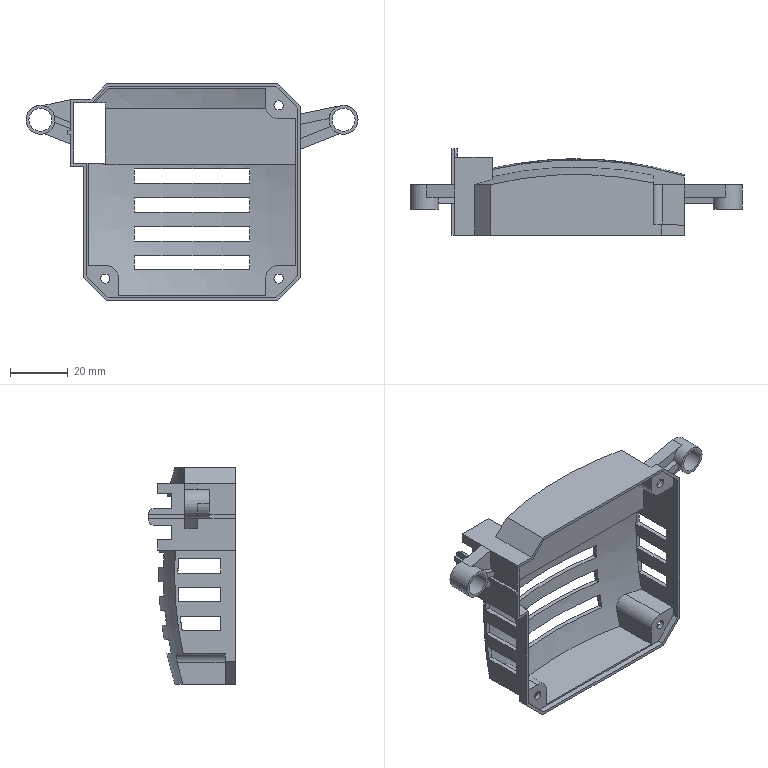Part | STEP file | HOUGAI_15_4 | 1 solid | 156 faces | box 115 x 30 x 75 mm | volume 16947 mm3 | plane 124 | cylinder 28 | sphere 4 | commonest cylinder face diameters 3.2 x6 8 x4 10 x4 6 x3 9 x3 4 x2